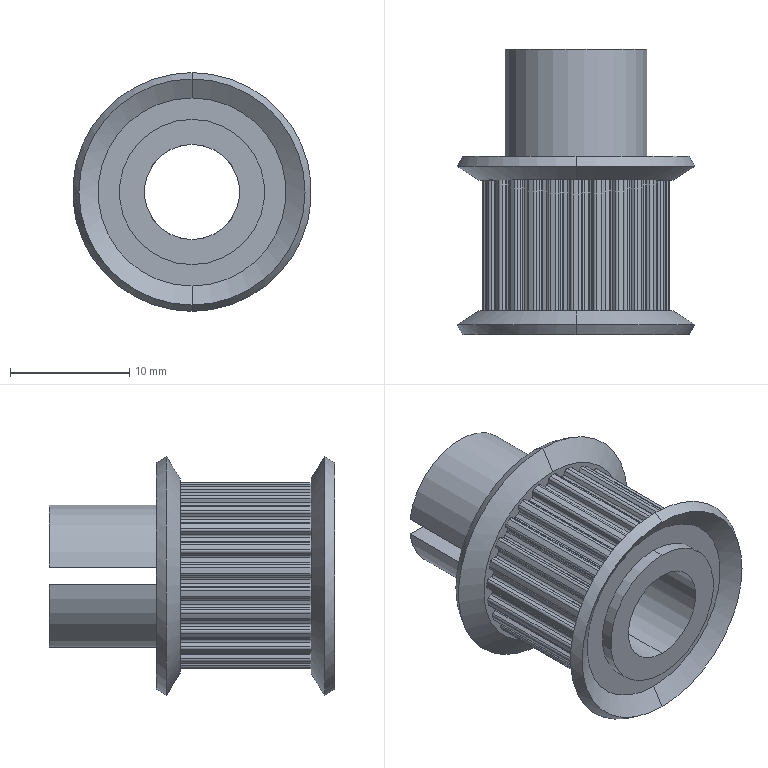Part | NX | features BREP 1 | 1 solid | 253 faces | box 20.061 x 24 x 20.061 mm | volume 2586 mm3 | cylinder 154 | plane 87 | cone 12 | commonest cylinder face diameters 0.46 x120 15.66 x25 12.2 x4 12 x3 8 x2